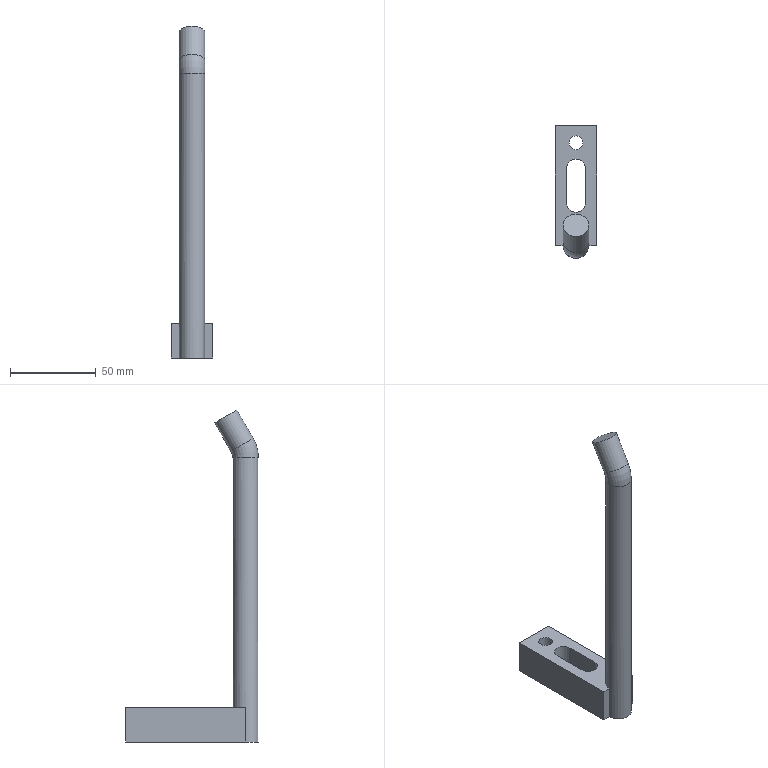Part | NX | features solid 2 | 1 solid | 16 faces | box 24 x 77.5 x 193.75 mm | volume 58617 mm3 | plane 10 | cylinder 5 | torus 1 | commonest cylinder face diameters 11 x2 15 x2 8 x1
STEP:
#1=CARTESIAN_POINT('',(75.,-47.96,5.));
#2=VERTEX_POINT('',#1);
#3=CARTESIAN_POINT('',(75.,-43.96,5.));
#4=DIRECTION('',(0.,0.,1.));
#5=DIRECTION('',(0.,-1.,0.));
#6=AXIS2_PLACEMENT_3D('',#3,#4,#5);
#7=CIRCLE('',#6,4.);
#8=EDGE_CURVE('',#2,#2,#7,.T.);
#9=ORIENTED_EDGE('',*,*,#8,.F.);
#10=EDGE_LOOP('',(#9));
#11=FACE_BOUND('',#10,.T.);
#12=CARTESIAN_POINT('',(80.5,-78.96,5.));
#13=VERTEX_POINT('',#12);
#14=CARTESIAN_POINT('',(80.5,-58.96,5.));
#15=VERTEX_POINT('',#14);
#16=CARTESIAN_POINT('',(80.5,-68.96,5.));
#17=DIRECTION('',(0.,1.,0.));
#18=VECTOR('',#17,1000.);
#19=LINE('',#16,#18);
#20=EDGE_CURVE('',#13,#15,#19,.T.);
#21=ORIENTED_EDGE('',*,*,#20,.F.);
#22=CARTESIAN_POINT('',(69.5,-78.96,5.));
#23=VERTEX_POINT('',#22);
#24=CARTESIAN_POINT('',(75.,-78.96,5.));
#25=DIRECTION('',(0.,0.,-1.));
#26=DIRECTION('',(0.,1.,0.));
#27=AXIS2_PLACEMENT_3D('',#24,#25,#26);
#28=CIRCLE('',#27,5.5);
#29=EDGE_CURVE('',#13,#23,#28,.T.);
#30=ORIENTED_EDGE('',*,*,#29,.T.);
#31=CARTESIAN_POINT('',(69.5,-58.96,5.));
#32=VERTEX_POINT('',#31);
#33=CARTESIAN_POINT('',(69.5,-68.96,5.));
#34=DIRECTION('',(0.,1.,0.));
#35=VECTOR('',#34,1000.);
#36=LINE('',#33,#35);
#37=EDGE_CURVE('',#23,#32,#36,.T.);
#38=ORIENTED_EDGE('',*,*,#37,.T.);
#39=CARTESIAN_POINT('',(75.,-58.96,5.));
#40=DIRECTION('',(0.,0.,-1.));
#41=DIRECTION('',(0.,1.,0.));
#42=AXIS2_PLACEMENT_3D('',#39,#40,#41);
#43=CIRCLE('',#42,5.5);
#44=EDGE_CURVE('',#32,#15,#43,.T.);
#45=ORIENTED_EDGE('',*,*,#44,.T.);
#46=EDGE_LOOP('',(#21,#30,#38,#45));
#47=FACE_BOUND('',#46,.T.);
#48=CARTESIAN_POINT('',(67.5,-103.96,5.));
#49=VERTEX_POINT('',#48);
#50=CARTESIAN_POINT('',(63.,-103.96,5.));
#51=VERTEX_POINT('',#50);
#52=CARTESIAN_POINT('',(87.,-103.96,5.));
#53=DIRECTION('',(-1.,0.,0.));
#54=VECTOR('',#53,1000.);
#55=LINE('',#52,#54);
#56=EDGE_CURVE('',#49,#51,#55,.T.);
#57=ORIENTED_EDGE('',*,*,#56,.F.);
#58=CARTESIAN_POINT('',(82.5,-103.96,5.));
#59=VERTEX_POINT('',#58);
#60=CARTESIAN_POINT('',(75.,-103.96,5.));
#61=DIRECTION('',(0.,0.,1.));
#62=DIRECTION('',(1.,0.,0.));
#63=AXIS2_PLACEMENT_3D('',#60,#61,#62);
#64=CIRCLE('',#63,7.5);
#65=EDGE_CURVE('',#49,#59,#64,.F.);
#66=ORIENTED_EDGE('',*,*,#65,.T.);
#67=CARTESIAN_POINT('',(87.,-103.96,5.));
#68=VERTEX_POINT('',#67);
#69=CARTESIAN_POINT('',(87.,-103.96,5.));
#70=DIRECTION('',(-1.,0.,0.));
#71=VECTOR('',#70,1000.);
#72=LINE('',#69,#71);
#73=EDGE_CURVE('',#68,#59,#72,.T.);
#74=ORIENTED_EDGE('',*,*,#73,.F.);
#75=CARTESIAN_POINT('',(87.,-33.96,5.));
#76=VERTEX_POINT('',#75);
#77=CARTESIAN_POINT('',(87.,-33.96,5.));
#78=DIRECTION('',(0.,-1.,0.));
#79=VECTOR('',#78,1000.);
#80=LINE('',#77,#79);
#81=EDGE_CURVE('',#76,#68,#80,.T.);
#82=ORIENTED_EDGE('',*,*,#81,.F.);
#83=CARTESIAN_POINT('',(63.,-33.96,5.));
#84=VERTEX_POINT('',#83);
#85=CARTESIAN_POINT('',(63.,-33.96,5.));
#86=DIRECTION('',(1.,0.,0.));
#87=VECTOR('',#86,1000.);
#88=LINE('',#85,#87);
#89=EDGE_CURVE('',#84,#76,#88,.T.);
#90=ORIENTED_EDGE('',*,*,#89,.F.);
#91=CARTESIAN_POINT('',(63.,-103.96,5.));
#92=DIRECTION('',(0.,1.,0.));
#93=VECTOR('',#92,1000.);
#94=LINE('',#91,#93);
#95=EDGE_CURVE('',#51,#84,#94,.T.);
#96=ORIENTED_EDGE('',*,*,#95,.F.);
#97=EDGE_LOOP('',(#57,#66,#74,#82,#90,#96));
#98=FACE_BOUND('',#97,.T.);
#99=CARTESIAN_POINT('',(87.,-33.96,5.));
#100=DIRECTION('',(0.,0.,1.));
#101=DIRECTION('',(0.,1.,0.));
#102=AXIS2_PLACEMENT_3D('',#99,#100,#101);
#103=PLANE('',#102);
#104=ADVANCED_FACE('',(#11,#47,#98),#103,.T.);
#105=CARTESIAN_POINT('',(67.5,-103.96,-15.));
#106=VERTEX_POINT('',#105);
#107=CARTESIAN_POINT('',(63.,-103.96,-15.));
#108=VERTEX_POINT('',#107);
#109=CARTESIAN_POINT('',(87.,-103.96,-15.));
#110=DIRECTION('',(-1.,0.,0.));
#111=VECTOR('',#110,1000.);
#112=LINE('',#109,#111);
#113=EDGE_CURVE('',#106,#108,#112,.T.);
#114=ORIENTED_EDGE('',*,*,#113,.T.);
#115=CARTESIAN_POINT('',(63.,-33.96,-15.));
#116=VERTEX_POINT('',#115);
#117=CARTESIAN_POINT('',(63.,-103.96,-15.));
#118=DIRECTION('',(0.,1.,0.));
#119=VECTOR('',#118,1000.);
#120=LINE('',#117,#119);
#121=EDGE_CURVE('',#108,#116,#120,.T.);
#122=ORIENTED_EDGE('',*,*,#121,.T.);
#123=CARTESIAN_POINT('',(87.,-33.96,-15.));
#124=VERTEX_POINT('',#123);
#125=CARTESIAN_POINT('',(63.,-33.96,-15.));
#126=DIRECTION('',(1.,0.,0.));
#127=VECTOR('',#126,1000.);
#128=LINE('',#125,#127);
#129=EDGE_CURVE('',#116,#124,#128,.T.);
#130=ORIENTED_EDGE('',*,*,#129,.T.);
#131=CARTESIAN_POINT('',(87.,-103.96,-15.));
#132=VERTEX_POINT('',#131);
#133=CARTESIAN_POINT('',(87.,-33.96,-15.));
#134=DIRECTION('',(0.,-1.,0.));
#135=VECTOR('',#134,1000.);
#136=LINE('',#133,#135);
#137=EDGE_CURVE('',#124,#132,#136,.T.);
#138=ORIENTED_EDGE('',*,*,#137,.T.);
#139=CARTESIAN_POINT('',(82.5,-103.96,-15.));
#140=VERTEX_POINT('',#139);
#141=CARTESIAN_POINT('',(87.,-103.96,-15.));
#142=DIRECTION('',(-1.,0.,0.));
#143=VECTOR('',#142,1000.);
#144=LINE('',#141,#143);
#145=EDGE_CURVE('',#132,#140,#144,.T.);
#146=ORIENTED_EDGE('',*,*,#145,.T.);
#147=CARTESIAN_POINT('',(75.,-103.96,-15.));
#148=DIRECTION('',(0.,0.,-1.));
#149=DIRECTION('',(0.,1.,0.));
#150=AXIS2_PLACEMENT_3D('',#147,#148,#149);
#151=CIRCLE('',#150,7.5);
#152=EDGE_CURVE('',#140,#106,#151,.T.);
#153=ORIENTED_EDGE('',*,*,#152,.T.);
#154=EDGE_LOOP('',(#114,#122,#130,#138,#146,#153));
#155=FACE_BOUND('',#154,.T.);
#156=CARTESIAN_POINT('',(69.5,-58.96,-15.));
#157=VERTEX_POINT('',#156);
#158=CARTESIAN_POINT('',(80.5,-58.96,-15.));
#159=VERTEX_POINT('',#158);
#160=CARTESIAN_POINT('',(75.,-58.96,-15.));
#161=DIRECTION('',(0.,0.,-1.));
#162=DIRECTION('',(0.,1.,0.));
#163=AXIS2_PLACEMENT_3D('',#160,#161,#162);
#164=CIRCLE('',#163,5.5);
#165=EDGE_CURVE('',#157,#159,#164,.T.);
#166=ORIENTED_EDGE('',*,*,#165,.F.);
#167=CARTESIAN_POINT('',(69.5,-78.96,-15.));
#168=VERTEX_POINT('',#167);
#169=CARTESIAN_POINT('',(69.5,-78.96,-15.));
#170=DIRECTION('',(0.,1.,0.));
#171=VECTOR('',#170,1000.);
#172=LINE('',#169,#171);
#173=EDGE_CURVE('',#168,#157,#172,.T.);
#174=ORIENTED_EDGE('',*,*,#173,.F.);
#175=CARTESIAN_POINT('',(80.5,-78.96,-15.));
#176=VERTEX_POINT('',#175);
#177=CARTESIAN_POINT('',(75.,-78.96,-15.));
#178=DIRECTION('',(0.,0.,-1.));
#179=DIRECTION('',(0.,1.,0.));
#180=AXIS2_PLACEMENT_3D('',#177,#178,#179);
#181=CIRCLE('',#180,5.5);
#182=EDGE_CURVE('',#176,#168,#181,.T.);
#183=ORIENTED_EDGE('',*,*,#182,.F.);
#184=CARTESIAN_POINT('',(80.5,-78.96,-15.));
#185=DIRECTION('',(0.,1.,0.));
#186=VECTOR('',#185,1000.);
#187=LINE('',#184,#186);
#188=EDGE_CURVE('',#176,#159,#187,.T.);
#189=ORIENTED_EDGE('',*,*,#188,.T.);
#190=EDGE_LOOP('',(#166,#174,#183,#189));
#191=FACE_BOUND('',#190,.T.);
#192=CARTESIAN_POINT('',(75.,-39.96,-15.));
#193=VERTEX_POINT('',#192);
#194=CARTESIAN_POINT('',(75.,-43.96,-15.));
#195=DIRECTION('',(0.,0.,-1.));
#196=DIRECTION('',(0.,1.,0.));
#197=AXIS2_PLACEMENT_3D('',#194,#195,#196);
#198=CIRCLE('',#197,4.);
#199=EDGE_CURVE('',#193,#193,#198,.T.);
#200=ORIENTED_EDGE('',*,*,#199,.F.);
#201=EDGE_LOOP('',(#200));
#202=FACE_BOUND('',#201,.T.);
#203=CARTESIAN_POINT('',(87.,-33.96,-15.));
#204=DIRECTION('',(0.,0.,1.));
#205=DIRECTION('',(0.,1.,0.));
#206=AXIS2_PLACEMENT_3D('',#203,#204,#205);
#207=PLANE('',#206);
#208=ADVANCED_FACE('',(#155,#191,#202),#207,.F.);
#209=ORIENTED_EDGE('',*,*,#137,.F.);
#210=CARTESIAN_POINT('',(87.,-33.96,5.));
#211=DIRECTION('',(0.,0.,-1.));
#212=VECTOR('',#211,1000.);
#213=LINE('',#210,#212);
#214=EDGE_CURVE('',#76,#124,#213,.T.);
#215=ORIENTED_EDGE('',*,*,#214,.F.);
#216=ORIENTED_EDGE('',*,*,#81,.T.);
#217=CARTESIAN_POINT('',(87.,-103.96,5.));
#218=DIRECTION('',(0.,0.,-1.));
#219=VECTOR('',#218,1000.);
#220=LINE('',#217,#219);
#221=EDGE_CURVE('',#68,#132,#220,.T.);
#222=ORIENTED_EDGE('',*,*,#221,.T.);
#223=EDGE_LOOP('',(#209,#215,#216,#222));
#224=FACE_BOUND('',#223,.T.);
#225=CARTESIAN_POINT('',(87.,-33.96,5.));
#226=DIRECTION('',(-1.,0.,0.));
#227=DIRECTION('',(0.,1.,0.));
#228=AXIS2_PLACEMENT_3D('',#225,#226,#227);
#229=PLANE('',#228);
#230=ADVANCED_FACE('',(#224),#229,.F.);
#231=ORIENTED_EDGE('',*,*,#129,.F.);
#232=CARTESIAN_POINT('',(63.,-33.96,5.));
#233=DIRECTION('',(0.,0.,-1.));
#234=VECTOR('',#233,1000.);
#235=LINE('',#232,#234);
#236=EDGE_CURVE('',#84,#116,#235,.T.);
#237=ORIENTED_EDGE('',*,*,#236,.F.);
#238=ORIENTED_EDGE('',*,*,#89,.T.);
#239=ORIENTED_EDGE('',*,*,#214,.T.);
#240=EDGE_LOOP('',(#231,#237,#238,#239));
#241=FACE_BOUND('',#240,.T.);
#242=CARTESIAN_POINT('',(63.,-33.96,5.));
#243=DIRECTION('',(0.,-1.,0.));
#244=DIRECTION('',(0.,0.,1.));
#245=AXIS2_PLACEMENT_3D('',#242,#243,#244);
#246=PLANE('',#245);
#247=ADVANCED_FACE('',(#241),#246,.F.);
#248=ORIENTED_EDGE('',*,*,#121,.F.);
#249=CARTESIAN_POINT('',(63.,-103.96,5.));
#250=DIRECTION('',(0.,0.,-1.));
#251=VECTOR('',#250,1000.);
#252=LINE('',#249,#251);
#253=EDGE_CURVE('',#51,#108,#252,.T.);
#254=ORIENTED_EDGE('',*,*,#253,.F.);
#255=ORIENTED_EDGE('',*,*,#95,.T.);
#256=ORIENTED_EDGE('',*,*,#236,.T.);
#257=EDGE_LOOP('',(#248,#254,#255,#256));
#258=FACE_BOUND('',#257,.T.);
#259=CARTESIAN_POINT('',(63.,-103.96,5.));
#260=DIRECTION('',(1.,0.,0.));
#261=DIRECTION('',(0.,-1.,0.));
#262=AXIS2_PLACEMENT_3D('',#259,#260,#261);
#263=PLANE('',#262);
#264=ADVANCED_FACE('',(#258),#263,.F.);
#265=CARTESIAN_POINT('',(67.5,-103.96,40.981));
#266=DIRECTION('',(0.,0.,-1.));
#267=VECTOR('',#266,1000.);
#268=LINE('',#265,#267);
#269=EDGE_CURVE('',#106,#49,#268,.F.);
#270=ORIENTED_EDGE('',*,*,#269,.T.);
#271=ORIENTED_EDGE('',*,*,#56,.T.);
#272=ORIENTED_EDGE('',*,*,#253,.T.);
#273=ORIENTED_EDGE('',*,*,#113,.F.);
#274=EDGE_LOOP('',(#270,#271,#272,#273));
#275=FACE_BOUND('',#274,.T.);
#276=CARTESIAN_POINT('',(87.,-103.96,5.));
#277=DIRECTION('',(0.,1.,0.));
#278=DIRECTION('',(0.,0.,-1.));
#279=AXIS2_PLACEMENT_3D('',#276,#277,#278);
#280=PLANE('',#279);
#281=ADVANCED_FACE('',(#275),#280,.F.);
#282=CARTESIAN_POINT('',(82.5,-103.96,40.981));
#283=DIRECTION('',(0.,0.,-1.));
#284=VECTOR('',#283,1000.);
#285=LINE('',#282,#284);
#286=EDGE_CURVE('',#59,#140,#285,.T.);
#287=ORIENTED_EDGE('',*,*,#286,.F.);
#288=ORIENTED_EDGE('',*,*,#65,.F.);
#289=ORIENTED_EDGE('',*,*,#269,.F.);
#290=ORIENTED_EDGE('',*,*,#152,.F.);
#291=EDGE_LOOP('',(#287,#288,#289,#290));
#292=FACE_BOUND('',#291,.T.);
#293=CARTESIAN_POINT('',(75.,-96.46,150.981));
#294=VERTEX_POINT('',#293);
#295=CARTESIAN_POINT('',(75.,-103.96,150.981));
#296=DIRECTION('',(0.,0.,-1.));
#297=DIRECTION('',(0.,1.,0.));
#298=AXIS2_PLACEMENT_3D('',#295,#296,#297);
#299=CIRCLE('',#298,7.5);
#300=EDGE_CURVE('',#294,#294,#299,.T.);
#301=ORIENTED_EDGE('',*,*,#300,.T.);
#302=EDGE_LOOP('',(#301));
#303=FACE_BOUND('',#302,.T.);
#304=CARTESIAN_POINT('',(75.,-103.96,40.981));
#305=DIRECTION('',(0.,0.,-1.));
#306=DIRECTION('',(0.,-1.,0.));
#307=AXIS2_PLACEMENT_3D('',#304,#305,#306);
#308=CYLINDRICAL_SURFACE('',#307,7.5);
#309=ADVANCED_FACE('',(#292,#303),#308,.T.);
#310=ORIENTED_EDGE('',*,*,#286,.T.);
#311=ORIENTED_EDGE('',*,*,#145,.F.);
#312=ORIENTED_EDGE('',*,*,#221,.F.);
#313=ORIENTED_EDGE('',*,*,#73,.T.);
#314=EDGE_LOOP('',(#310,#311,#312,#313));
#315=FACE_BOUND('',#314,.T.);
#316=CARTESIAN_POINT('',(87.,-103.96,5.));
#317=DIRECTION('',(0.,1.,0.));
#318=DIRECTION('',(0.,0.,-1.));
#319=AXIS2_PLACEMENT_3D('',#316,#317,#318);
#320=PLANE('',#319);
#321=ADVANCED_FACE('',(#315),#320,.F.);
#322=ORIENTED_EDGE('',*,*,#8,.T.);
#323=EDGE_LOOP('',(#322));
#324=FACE_BOUND('',#323,.T.);
#325=ORIENTED_EDGE('',*,*,#199,.T.);
#326=EDGE_LOOP('',(#325));
#327=FACE_BOUND('',#326,.T.);
#328=CARTESIAN_POINT('',(75.,-43.96,5.));
#329=DIRECTION('',(0.,0.,-1.));
#330=DIRECTION('',(0.,-1.,0.));
#331=AXIS2_PLACEMENT_3D('',#328,#329,#330);
#332=CYLINDRICAL_SURFACE('',#331,4.);
#333=ADVANCED_FACE('',(#324,#327),#332,.F.);
#334=ORIENTED_EDGE('',*,*,#29,.F.);
#335=CARTESIAN_POINT('',(80.5,-78.96,5.));
#336=DIRECTION('',(0.,0.,1.));
#337=VECTOR('',#336,1000.);
#338=LINE('',#335,#337);
#339=EDGE_CURVE('',#176,#13,#338,.T.);
#340=ORIENTED_EDGE('',*,*,#339,.F.);
#341=ORIENTED_EDGE('',*,*,#182,.T.);
#342=CARTESIAN_POINT('',(69.5,-78.96,5.));
#343=DIRECTION('',(0.,0.,1.));
#344=VECTOR('',#343,1000.);
#345=LINE('',#342,#344);
#346=EDGE_CURVE('',#168,#23,#345,.T.);
#347=ORIENTED_EDGE('',*,*,#346,.T.);
#348=EDGE_LOOP('',(#334,#340,#341,#347));
#349=FACE_BOUND('',#348,.T.);
#350=CARTESIAN_POINT('',(75.,-78.96,5.));
#351=DIRECTION('',(0.,0.,1.));
#352=DIRECTION('',(0.,1.,0.));
#353=AXIS2_PLACEMENT_3D('',#350,#351,#352);
#354=CYLINDRICAL_SURFACE('',#353,5.5);
#355=ADVANCED_FACE('',(#349),#354,.F.);
#356=ORIENTED_EDGE('',*,*,#37,.F.);
#357=ORIENTED_EDGE('',*,*,#346,.F.);
#358=ORIENTED_EDGE('',*,*,#173,.T.);
#359=CARTESIAN_POINT('',(69.5,-58.96,5.));
#360=DIRECTION('',(0.,0.,1.));
#361=VECTOR('',#360,1000.);
#362=LINE('',#359,#361);
#363=EDGE_CURVE('',#157,#32,#362,.T.);
#364=ORIENTED_EDGE('',*,*,#363,.T.);
#365=EDGE_LOOP('',(#356,#357,#358,#364));
#366=FACE_BOUND('',#365,.T.);
#367=CARTESIAN_POINT('',(69.5,-68.96,5.));
#368=DIRECTION('',(-1.,0.,0.));
#369=DIRECTION('',(0.,0.,-1.));
#370=AXIS2_PLACEMENT_3D('',#367,#368,#369);
#371=PLANE('',#370);
#372=ADVANCED_FACE('',(#366),#371,.F.);
#373=ORIENTED_EDGE('',*,*,#44,.F.);
#374=ORIENTED_EDGE('',*,*,#363,.F.);
#375=ORIENTED_EDGE('',*,*,#165,.T.);
#376=CARTESIAN_POINT('',(80.5,-58.96,5.));
#377=DIRECTION('',(0.,0.,1.));
#378=VECTOR('',#377,1000.);
#379=LINE('',#376,#378);
#380=EDGE_CURVE('',#159,#15,#379,.T.);
#381=ORIENTED_EDGE('',*,*,#380,.T.);
#382=EDGE_LOOP('',(#373,#374,#375,#381));
#383=FACE_BOUND('',#382,.T.);
#384=CARTESIAN_POINT('',(75.,-58.96,5.));
#385=DIRECTION('',(0.,0.,1.));
#386=DIRECTION('',(0.,1.,0.));
#387=AXIS2_PLACEMENT_3D('',#384,#385,#386);
#388=CYLINDRICAL_SURFACE('',#387,5.5);
#389=ADVANCED_FACE('',(#383),#388,.F.);
#390=ORIENTED_EDGE('',*,*,#20,.T.);
#391=ORIENTED_EDGE('',*,*,#380,.F.);
#392=ORIENTED_EDGE('',*,*,#188,.F.);
#393=ORIENTED_EDGE('',*,*,#339,.T.);
#394=EDGE_LOOP('',(#390,#391,#392,#393));
#395=FACE_BOUND('',#394,.T.);
#396=CARTESIAN_POINT('',(80.5,-68.96,5.));
#397=DIRECTION('',(1.,0.,0.));
#398=DIRECTION('',(0.,0.,1.));
#399=AXIS2_PLACEMENT_3D('',#396,#397,#398);
#400=PLANE('',#399);
#401=ADVANCED_FACE('',(#395),#400,.F.);
#402=CARTESIAN_POINT('',(75.,-95.455,154.731));
#403=VERTEX_POINT('',#402);
#404=CARTESIAN_POINT('',(75.,-101.951,158.481));
#405=DIRECTION('',(0.,-0.5,-0.866));
#406=DIRECTION('',(0.,0.866,-0.5));
#407=AXIS2_PLACEMENT_3D('',#404,#405,#406);
#408=CIRCLE('',#407,7.5);
#409=EDGE_CURVE('',#403,#403,#408,.T.);
#410=ORIENTED_EDGE('',*,*,#409,.F.);
#411=EDGE_LOOP('',(#410));
#412=FACE_BOUND('',#411,.T.);
#413=CARTESIAN_POINT('',(75.,-85.918,171.25));
#414=VERTEX_POINT('',#413);
#415=CARTESIAN_POINT('',(75.,-92.413,175.));
#416=DIRECTION('',(0.,-0.5,-0.866));
#417=DIRECTION('',(0.,0.866,-0.5));
#418=AXIS2_PLACEMENT_3D('',#415,#416,#417);
#419=CIRCLE('',#418,7.5);
#420=EDGE_CURVE('',#414,#414,#419,.T.);
#421=ORIENTED_EDGE('',*,*,#420,.T.);
#422=EDGE_LOOP('',(#421));
#423=FACE_BOUND('',#422,.T.);
#424=CARTESIAN_POINT('',(75.,-101.951,158.481));
#425=DIRECTION('',(0.,0.5,0.866));
#426=DIRECTION('',(0.,0.866,-0.5));
#427=AXIS2_PLACEMENT_3D('',#424,#425,#426);
#428=CYLINDRICAL_SURFACE('',#427,7.5);
#429=ADVANCED_FACE('',(#412,#423),#428,.T.);
#430=ORIENTED_EDGE('',*,*,#300,.F.);
#431=EDGE_LOOP('',(#430));
#432=FACE_BOUND('',#431,.T.);
#433=ORIENTED_EDGE('',*,*,#409,.T.);
#434=EDGE_LOOP('',(#433));
#435=FACE_BOUND('',#434,.T.);
#436=CARTESIAN_POINT('',(75.,-88.96,150.981));
#437=DIRECTION('',(1.,0.,0.));
#438=DIRECTION('',(0.,0.,1.));
#439=AXIS2_PLACEMENT_3D('',#436,#437,#438);
#440=TOROIDAL_SURFACE('',#439,15.,7.5);
#441=ADVANCED_FACE('',(#432,#435),#440,.T.);
#442=ORIENTED_EDGE('',*,*,#420,.F.);
#443=EDGE_LOOP('',(#442));
#444=FACE_BOUND('',#443,.T.);
#445=CARTESIAN_POINT('',(75.,-92.413,175.));
#446=DIRECTION('',(0.,0.5,0.866));
#447=DIRECTION('',(0.,0.866,-0.5));
#448=AXIS2_PLACEMENT_3D('',#445,#446,#447);
#449=PLANE('',#448);
#450=ADVANCED_FACE('',(#444),#449,.T.);
#451=CLOSED_SHELL('',(#104,#208,#230,#247,#264,#281,#309,#321,#333,#355,#372,#389,#401,#429,#441,#450));
#452=MANIFOLD_SOLID_BREP('',#451);
#453=(LENGTH_UNIT()NAMED_UNIT(*)SI_UNIT(.MILLI.,.METRE.));
#454=UNCERTAINTY_MEASURE_WITH_UNIT(LENGTH_MEASURE(0.00001),#453,'','');
#455=(NAMED_UNIT(*)PLANE_ANGLE_UNIT()SI_UNIT($,.RADIAN.));
#456=(NAMED_UNIT(*)SI_UNIT($,.STERADIAN.)SOLID_ANGLE_UNIT());
#457=(GEOMETRIC_REPRESENTATION_CONTEXT(3)GLOBAL_UNCERTAINTY_ASSIGNED_CONTEXT((#454))GLOBAL_UNIT_ASSIGNED_CONTEXT((#453,#455,#456))REPRESENTATION_CONTEXT('',''));
#458=ADVANCED_BREP_SHAPE_REPRESENTATION('',(#452),#457);